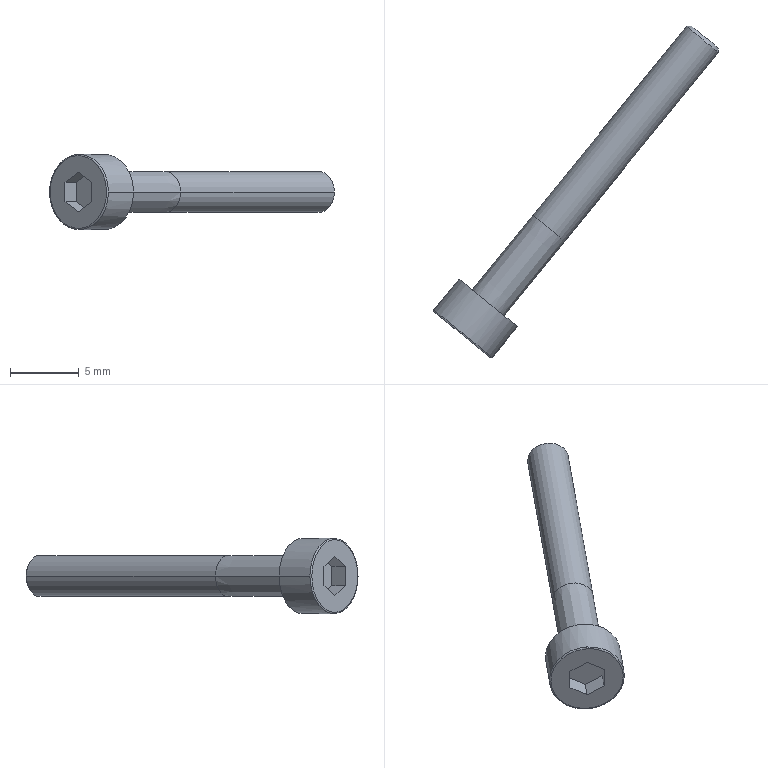Part | SolidWorks | features BaseBody 1 | 1 solid | 20 faces | box 20.765 x 24.207 x 5.5 mm | volume 240.606 mm3 | plane 10 | cylinder 4 | cone 4 | spline 2 | commonest cylinder face diameters 3 x2 5.5 x2
STEP:
#1=CARTESIAN_POINT('',(523.564,-199.626,281.731));
#2=VERTEX_POINT('',#1);
#3=CARTESIAN_POINT('',(525.697,-201.361,278.981));
#4=VERTEX_POINT('',#3);
#5=CARTESIAN_POINT('',(523.564,-199.626,278.981));
#6=DIRECTION('',(0.6309,0.7758,-0.000000012));
#7=DIRECTION('',(-0.7758,0.6309,0.));
#8=AXIS2_PLACEMENT_3D('',#5,#6,#7);
#9=CIRCLE('',#8,2.75);
#10=EDGE_CURVE('',#2,#4,#9,.T.);
#11=ORIENTED_EDGE('',*,*,#10,.F.);
#12=CARTESIAN_POINT('',(523.5,-199.704,281.631));
#13=VERTEX_POINT('',#12);
#14=CARTESIAN_POINT('',(523.564,-199.626,281.631));
#15=DIRECTION('',(0.7758,-0.6309,-0.000000021));
#16=DIRECTION('',(0.000000024,-0.000000004,1.));
#17=AXIS2_PLACEMENT_3D('',#14,#15,#16);
#18=CIRCLE('',#17,0.1);
#19=EDGE_CURVE('',#2,#13,#18,.T.);
#20=ORIENTED_EDGE('',*,*,#19,.T.);
#21=CARTESIAN_POINT('',(523.5,-199.704,276.331));
#22=VERTEX_POINT('',#21);
#23=CARTESIAN_POINT('',(523.5,-199.704,281.631));
#24=CARTESIAN_POINT('',(527.612,-203.048,281.631));
#25=CARTESIAN_POINT('',(527.612,-203.048,276.331));
#26=CARTESIAN_POINT('',(523.5,-199.704,276.331));
#27=(BOUNDED_CURVE()B_SPLINE_CURVE(3,(#23,#24,#25,#26),.UNSPECIFIED.,.F.,.F.)B_SPLINE_CURVE_WITH_KNOTS((4,4),(0.,1.),.UNSPECIFIED.)CURVE()GEOMETRIC_REPRESENTATION_ITEM()RATIONAL_B_SPLINE_CURVE((1.,0.3333,0.3333,1.))REPRESENTATION_ITEM(''));
#28=EDGE_CURVE('',#13,#22,#27,.T.);
#29=ORIENTED_EDGE('',*,*,#28,.T.);
#30=CARTESIAN_POINT('',(523.564,-199.626,276.231));
#31=VERTEX_POINT('',#30);
#32=CARTESIAN_POINT('',(523.564,-199.626,276.331));
#33=DIRECTION('',(-0.7758,0.6309,0.000000021));
#34=DIRECTION('',(-0.000000024,0.000000004,-1.));
#35=AXIS2_PLACEMENT_3D('',#32,#33,#34);
#36=CIRCLE('',#35,0.1);
#37=EDGE_CURVE('',#31,#22,#36,.T.);
#38=ORIENTED_EDGE('',*,*,#37,.F.);
#39=CARTESIAN_POINT('',(523.564,-199.626,278.981));
#40=DIRECTION('',(0.6309,0.7758,-0.000000012));
#41=DIRECTION('',(-0.7758,0.6309,0.));
#42=AXIS2_PLACEMENT_3D('',#39,#40,#41);
#43=CIRCLE('',#42,2.75);
#44=EDGE_CURVE('',#4,#31,#43,.T.);
#45=ORIENTED_EDGE('',*,*,#44,.F.);
#46=EDGE_LOOP('',(#11,#20,#29,#38,#45));
#47=FACE_OUTER_BOUND('',#46,.T.);
#48=CARTESIAN_POINT('',(523.564,-199.626,281.731));
#49=CARTESIAN_POINT('',(527.831,-203.097,281.731));
#50=CARTESIAN_POINT('',(527.831,-203.097,276.231));
#51=CARTESIAN_POINT('',(523.564,-199.626,276.231));
#52=CARTESIAN_POINT('',(523.527,-199.672,281.731));
#53=CARTESIAN_POINT('',(527.794,-203.142,281.731));
#54=CARTESIAN_POINT('',(527.794,-203.142,276.231));
#55=CARTESIAN_POINT('',(523.527,-199.672,276.231));
#56=CARTESIAN_POINT('',(523.5,-199.704,281.689));
#57=CARTESIAN_POINT('',(527.703,-203.122,281.689));
#58=CARTESIAN_POINT('',(527.703,-203.122,276.272));
#59=CARTESIAN_POINT('',(523.5,-199.704,276.272));
#60=CARTESIAN_POINT('',(523.5,-199.704,281.631));
#61=CARTESIAN_POINT('',(527.612,-203.048,281.631));
#62=CARTESIAN_POINT('',(527.612,-203.048,276.331));
#63=CARTESIAN_POINT('',(523.5,-199.704,276.331));
#64=(BOUNDED_SURFACE()B_SPLINE_SURFACE(3,3,((#48,#49,#50,#51),(#52,#53,#54,#55),(#56,#57,#58,#59),(#60,#61,#62,#63)),.UNSPECIFIED.,.F.,.F.,.T.)B_SPLINE_SURFACE_WITH_KNOTS((4,4),(4,4),(0.,1.),(0.,1.),.UNSPECIFIED.)GEOMETRIC_REPRESENTATION_ITEM()RATIONAL_B_SPLINE_SURFACE(((1.,0.3333,0.3333,1.),(0.8047,0.2682,0.2682,0.8047),(0.8047,0.2682,0.2682,0.8047),(1.,0.3333,0.3333,1.)))REPRESENTATION_ITEM('')SURFACE());
#65=ADVANCED_FACE('',(#47),#64,.T.);
#66=CARTESIAN_POINT('',(528.646,-190.999,278.981));
#67=VERTEX_POINT('',#66);
#68=CARTESIAN_POINT('',(530.974,-192.892,278.981));
#69=VERTEX_POINT('',#68);
#70=CARTESIAN_POINT('',(529.81,-191.946,278.981));
#71=DIRECTION('',(0.6309,0.7758,-0.000000012));
#72=DIRECTION('',(-0.7758,0.6309,0.));
#73=AXIS2_PLACEMENT_3D('',#70,#71,#72);
#74=CIRCLE('',#73,1.5);
#75=EDGE_CURVE('',#67,#69,#74,.T.);
#76=ORIENTED_EDGE('',*,*,#75,.T.);
#77=CARTESIAN_POINT('',(542.173,-179.121,278.981));
#78=VERTEX_POINT('',#77);
#79=CARTESIAN_POINT('',(536.573,-186.006,278.981));
#80=DIRECTION('',(0.6309,0.7758,-0.000000012));
#81=VECTOR('',#80,1000.);
#82=LINE('',#79,#81);
#83=EDGE_CURVE('',#69,#78,#82,.T.);
#84=ORIENTED_EDGE('',*,*,#83,.T.);
#85=CARTESIAN_POINT('',(539.845,-177.228,278.981));
#86=VERTEX_POINT('',#85);
#87=CARTESIAN_POINT('',(541.009,-178.174,278.981));
#88=DIRECTION('',(-0.6309,-0.7758,0.000000012));
#89=DIRECTION('',(-0.7758,0.6309,0.));
#90=AXIS2_PLACEMENT_3D('',#87,#88,#89);
#91=CIRCLE('',#90,1.5);
#92=EDGE_CURVE('',#78,#86,#91,.T.);
#93=ORIENTED_EDGE('',*,*,#92,.T.);
#94=CARTESIAN_POINT('',(534.246,-184.114,278.981));
#95=DIRECTION('',(0.6309,0.7758,-0.000000012));
#96=VECTOR('',#95,1000.);
#97=LINE('',#94,#96);
#98=EDGE_CURVE('',#67,#86,#97,.T.);
#99=ORIENTED_EDGE('',*,*,#98,.F.);
#100=EDGE_LOOP('',(#76,#84,#93,#99));
#101=FACE_OUTER_BOUND('',#100,.T.);
#102=CARTESIAN_POINT('',(535.409,-185.06,278.981));
#103=DIRECTION('',(0.6309,0.7758,-0.000000012));
#104=DIRECTION('',(-0.7758,0.6309,0.));
#105=AXIS2_PLACEMENT_3D('',#102,#103,#104);
#106=CYLINDRICAL_SURFACE('',#105,1.5);
#107=ADVANCED_FACE('',(#101),#106,.T.);
#108=CARTESIAN_POINT('',(542.136,-178.769,278.981));
#109=VERTEX_POINT('',#108);
#110=CARTESIAN_POINT('',(540.197,-177.192,278.981));
#111=VERTEX_POINT('',#110);
#112=CARTESIAN_POINT('',(541.167,-177.98,278.981));
#113=DIRECTION('',(-0.6309,-0.7758,0.000000012));
#114=DIRECTION('',(0.7758,-0.6309,0.));
#115=AXIS2_PLACEMENT_3D('',#112,#113,#114);
#116=CIRCLE('',#115,1.25);
#117=EDGE_CURVE('',#109,#111,#116,.T.);
#118=ORIENTED_EDGE('',*,*,#117,.T.);
#119=CARTESIAN_POINT('',(539.845,-177.228,278.981));
#120=DIRECTION('',(-0.9947,-0.1025,0.000000009));
#121=VECTOR('',#120,1000.);
#122=LINE('',#119,#121);
#123=EDGE_CURVE('',#111,#86,#122,.T.);
#124=ORIENTED_EDGE('',*,*,#123,.T.);
#125=ORIENTED_EDGE('',*,*,#92,.F.);
#126=CARTESIAN_POINT('',(542.173,-179.121,278.981));
#127=DIRECTION('',(0.1025,-0.9947,0.000000009));
#128=VECTOR('',#127,1000.);
#129=LINE('',#126,#128);
#130=EDGE_CURVE('',#109,#78,#129,.T.);
#131=ORIENTED_EDGE('',*,*,#130,.F.);
#132=EDGE_LOOP('',(#118,#124,#125,#131));
#133=FACE_OUTER_BOUND('',#132,.T.);
#134=CARTESIAN_POINT('',(541.009,-178.174,278.981));
#135=DIRECTION('',(-0.6309,-0.7758,0.000000012));
#136=DIRECTION('',(0.7758,-0.6309,0.));
#137=AXIS2_PLACEMENT_3D('',#134,#135,#136);
#138=CONICAL_SURFACE('',#137,1.5,0.7854);
#139=ADVANCED_FACE('',(#133),#138,.T.);
#140=CARTESIAN_POINT('',(524.23,-196.431,278.981));
#141=VERTEX_POINT('',#140);
#142=CARTESIAN_POINT('',(526.556,-198.322,278.981));
#143=VERTEX_POINT('',#142);
#144=CARTESIAN_POINT('',(525.393,-197.376,278.981));
#145=DIRECTION('',(0.6309,0.7758,-0.000000012));
#146=DIRECTION('',(-0.7758,0.6309,0.));
#147=AXIS2_PLACEMENT_3D('',#144,#145,#146);
#148=CIRCLE('',#147,1.499);
#149=EDGE_CURVE('',#141,#143,#148,.T.);
#150=ORIENTED_EDGE('',*,*,#149,.T.);
#151=CARTESIAN_POINT('',(530.974,-192.892,278.981));
#152=DIRECTION('',(0.631,0.7758,-0.000000012));
#153=VECTOR('',#152,1000.);
#154=LINE('',#151,#153);
#155=EDGE_CURVE('',#143,#69,#154,.T.);
#156=ORIENTED_EDGE('',*,*,#155,.T.);
#157=ORIENTED_EDGE('',*,*,#75,.F.);
#158=CARTESIAN_POINT('',(528.646,-190.999,278.981));
#159=DIRECTION('',(0.6308,0.7759,-0.000000012));
#160=VECTOR('',#159,1000.);
#161=LINE('',#158,#160);
#162=EDGE_CURVE('',#141,#67,#161,.T.);
#163=ORIENTED_EDGE('',*,*,#162,.F.);
#164=EDGE_LOOP('',(#150,#156,#157,#163));
#165=FACE_OUTER_BOUND('',#164,.T.);
#166=CARTESIAN_POINT('',(529.81,-191.946,278.981));
#167=DIRECTION('',(0.6309,0.7758,-0.000000012));
#168=DIRECTION('',(-0.7758,0.6309,0.));
#169=AXIS2_PLACEMENT_3D('',#166,#167,#168);
#170=CONICAL_SURFACE('',#169,1.5,0.0001071);
#171=ADVANCED_FACE('',(#165),#170,.T.);
#172=CARTESIAN_POINT('',(521.43,-197.891,278.981));
#173=VERTEX_POINT('',#172);
#174=CARTESIAN_POINT('',(523.564,-199.626,278.981));
#175=DIRECTION('',(0.6309,0.7758,-0.000000012));
#176=DIRECTION('',(-0.7758,0.6309,0.));
#177=AXIS2_PLACEMENT_3D('',#174,#175,#176);
#178=CIRCLE('',#177,2.75);
#179=EDGE_CURVE('',#173,#2,#178,.T.);
#180=ORIENTED_EDGE('',*,*,#179,.T.);
#181=ORIENTED_EDGE('',*,*,#10,.T.);
#182=CARTESIAN_POINT('',(527.527,-199.112,278.981));
#183=VERTEX_POINT('',#182);
#184=CARTESIAN_POINT('',(526.612,-200.236,278.981));
#185=DIRECTION('',(0.6309,0.7758,-0.000000012));
#186=VECTOR('',#185,1000.);
#187=LINE('',#184,#186);
#188=EDGE_CURVE('',#4,#183,#187,.T.);
#189=ORIENTED_EDGE('',*,*,#188,.T.);
#190=CARTESIAN_POINT('',(523.26,-195.641,278.981));
#191=VERTEX_POINT('',#190);
#192=CARTESIAN_POINT('',(525.393,-197.376,278.981));
#193=DIRECTION('',(0.6309,0.7758,-0.000000012));
#194=DIRECTION('',(-0.7758,0.6309,0.));
#195=AXIS2_PLACEMENT_3D('',#192,#193,#194);
#196=CIRCLE('',#195,2.75);
#197=EDGE_CURVE('',#191,#183,#196,.T.);
#198=ORIENTED_EDGE('',*,*,#197,.F.);
#199=CARTESIAN_POINT('',(522.345,-196.766,278.981));
#200=DIRECTION('',(0.6309,0.7758,-0.000000012));
#201=VECTOR('',#200,1000.);
#202=LINE('',#199,#201);
#203=EDGE_CURVE('',#173,#191,#202,.T.);
#204=ORIENTED_EDGE('',*,*,#203,.F.);
#205=EDGE_LOOP('',(#180,#181,#189,#198,#204));
#206=FACE_OUTER_BOUND('',#205,.T.);
#207=CARTESIAN_POINT('',(524.478,-198.501,278.981));
#208=DIRECTION('',(0.6309,0.7758,-0.000000012));
#209=DIRECTION('',(-0.7758,0.6309,0.));
#210=AXIS2_PLACEMENT_3D('',#207,#208,#209);
#211=CYLINDRICAL_SURFACE('',#210,2.75);
#212=ADVANCED_FACE('',(#206),#211,.T.);
#213=ORIENTED_EDGE('',*,*,#83,.F.);
#214=CARTESIAN_POINT('',(529.81,-191.946,278.981));
#215=DIRECTION('',(0.6309,0.7758,-0.000000012));
#216=DIRECTION('',(-0.7758,0.6309,0.));
#217=AXIS2_PLACEMENT_3D('',#214,#215,#216);
#218=CIRCLE('',#217,1.5);
#219=EDGE_CURVE('',#69,#67,#218,.T.);
#220=ORIENTED_EDGE('',*,*,#219,.T.);
#221=ORIENTED_EDGE('',*,*,#98,.T.);
#222=CARTESIAN_POINT('',(541.009,-178.174,278.981));
#223=DIRECTION('',(-0.6309,-0.7758,0.000000012));
#224=DIRECTION('',(-0.7758,0.6309,0.));
#225=AXIS2_PLACEMENT_3D('',#222,#223,#224);
#226=CIRCLE('',#225,1.5);
#227=EDGE_CURVE('',#86,#78,#226,.T.);
#228=ORIENTED_EDGE('',*,*,#227,.T.);
#229=EDGE_LOOP('',(#213,#220,#221,#228));
#230=FACE_OUTER_BOUND('',#229,.T.);
#231=CARTESIAN_POINT('',(535.409,-185.06,278.981));
#232=DIRECTION('',(0.6309,0.7758,-0.000000012));
#233=DIRECTION('',(-0.7758,0.6309,0.));
#234=AXIS2_PLACEMENT_3D('',#231,#232,#233);
#235=CYLINDRICAL_SURFACE('',#234,1.5);
#236=ADVANCED_FACE('',(#230),#235,.T.);
#237=ORIENTED_EDGE('',*,*,#123,.F.);
#238=CARTESIAN_POINT('',(541.167,-177.98,278.981));
#239=DIRECTION('',(-0.6309,-0.7758,0.000000012));
#240=DIRECTION('',(0.7758,-0.6309,0.));
#241=AXIS2_PLACEMENT_3D('',#238,#239,#240);
#242=CIRCLE('',#241,1.25);
#243=EDGE_CURVE('',#111,#109,#242,.T.);
#244=ORIENTED_EDGE('',*,*,#243,.T.);
#245=ORIENTED_EDGE('',*,*,#130,.T.);
#246=ORIENTED_EDGE('',*,*,#227,.F.);
#247=EDGE_LOOP('',(#237,#244,#245,#246));
#248=FACE_OUTER_BOUND('',#247,.T.);
#249=CARTESIAN_POINT('',(541.009,-178.174,278.981));
#250=DIRECTION('',(-0.6309,-0.7758,0.000000012));
#251=DIRECTION('',(0.7758,-0.6309,0.));
#252=AXIS2_PLACEMENT_3D('',#249,#250,#251);
#253=CONICAL_SURFACE('',#252,1.5,0.7854);
#254=ADVANCED_FACE('',(#248),#253,.T.);
#255=ORIENTED_EDGE('',*,*,#155,.F.);
#256=CARTESIAN_POINT('',(525.393,-197.376,278.981));
#257=DIRECTION('',(0.6309,0.7758,-0.000000012));
#258=DIRECTION('',(-0.7758,0.6309,0.));
#259=AXIS2_PLACEMENT_3D('',#256,#257,#258);
#260=CIRCLE('',#259,1.499);
#261=EDGE_CURVE('',#143,#141,#260,.T.);
#262=ORIENTED_EDGE('',*,*,#261,.T.);
#263=ORIENTED_EDGE('',*,*,#162,.T.);
#264=ORIENTED_EDGE('',*,*,#219,.F.);
#265=EDGE_LOOP('',(#255,#262,#263,#264));
#266=FACE_OUTER_BOUND('',#265,.T.);
#267=CARTESIAN_POINT('',(529.81,-191.946,278.981));
#268=DIRECTION('',(0.6309,0.7758,-0.000000012));
#269=DIRECTION('',(-0.7758,0.6309,0.));
#270=AXIS2_PLACEMENT_3D('',#267,#268,#269);
#271=CONICAL_SURFACE('',#270,1.5,0.0001071);
#272=ADVANCED_FACE('',(#266),#271,.T.);
#273=ORIENTED_EDGE('',*,*,#117,.F.);
#274=ORIENTED_EDGE('',*,*,#243,.F.);
#275=EDGE_LOOP('',(#273,#274));
#276=FACE_OUTER_BOUND('',#275,.T.);
#277=CARTESIAN_POINT('',(541.167,-177.98,278.356));
#278=DIRECTION('',(0.6309,0.7758,-0.000000012));
#279=DIRECTION('',(-0.7758,0.6309,0.));
#280=AXIS2_PLACEMENT_3D('',#277,#278,#279);
#281=PLANE('',#280);
#282=ADVANCED_FACE('',(#276),#281,.T.);
#283=ORIENTED_EDGE('',*,*,#149,.F.);
#284=ORIENTED_EDGE('',*,*,#261,.F.);
#285=EDGE_LOOP('',(#283,#284));
#286=FACE_BOUND('',#285,.T.);
#287=ORIENTED_EDGE('',*,*,#197,.T.);
#288=CARTESIAN_POINT('',(525.393,-197.376,278.981));
#289=DIRECTION('',(0.6309,0.7758,-0.000000012));
#290=DIRECTION('',(-0.7758,0.6309,0.));
#291=AXIS2_PLACEMENT_3D('',#288,#289,#290);
#292=CIRCLE('',#291,2.75);
#293=EDGE_CURVE('',#183,#191,#292,.T.);
#294=ORIENTED_EDGE('',*,*,#293,.T.);
#295=EDGE_LOOP('',(#287,#294));
#296=FACE_OUTER_BOUND('',#295,.T.);
#297=CARTESIAN_POINT('',(525.393,-197.376,277.606));
#298=DIRECTION('',(0.6309,0.7758,-0.000000012));
#299=DIRECTION('',(-0.7758,0.6309,0.));
#300=AXIS2_PLACEMENT_3D('',#297,#298,#299);
#301=PLANE('',#300);
#302=ADVANCED_FACE('',(#286,#296),#301,.T.);
#303=ORIENTED_EDGE('',*,*,#188,.F.);
#304=ORIENTED_EDGE('',*,*,#44,.T.);
#305=CARTESIAN_POINT('',(523.564,-199.626,278.981));
#306=DIRECTION('',(0.6309,0.7758,-0.000000012));
#307=DIRECTION('',(-0.7758,0.6309,0.));
#308=AXIS2_PLACEMENT_3D('',#305,#306,#307);
#309=CIRCLE('',#308,2.75);
#310=EDGE_CURVE('',#31,#173,#309,.T.);
#311=ORIENTED_EDGE('',*,*,#310,.T.);
#312=ORIENTED_EDGE('',*,*,#203,.T.);
#313=ORIENTED_EDGE('',*,*,#293,.F.);
#314=EDGE_LOOP('',(#303,#304,#311,#312,#313));
#315=FACE_OUTER_BOUND('',#314,.T.);
#316=CARTESIAN_POINT('',(524.478,-198.501,278.981));
#317=DIRECTION('',(0.6309,0.7758,-0.000000012));
#318=DIRECTION('',(-0.7758,0.6309,0.));
#319=AXIS2_PLACEMENT_3D('',#316,#317,#318);
#320=CYLINDRICAL_SURFACE('',#319,2.75);
#321=ADVANCED_FACE('',(#315),#320,.T.);
#322=ORIENTED_EDGE('',*,*,#19,.F.);
#323=ORIENTED_EDGE('',*,*,#179,.F.);
#324=ORIENTED_EDGE('',*,*,#310,.F.);
#325=ORIENTED_EDGE('',*,*,#37,.T.);
#326=CARTESIAN_POINT('',(523.5,-199.704,276.331));
#327=CARTESIAN_POINT('',(519.389,-196.36,276.331));
#328=CARTESIAN_POINT('',(519.389,-196.36,281.631));
#329=CARTESIAN_POINT('',(523.5,-199.704,281.631));
#330=(BOUNDED_CURVE()B_SPLINE_CURVE(3,(#326,#327,#328,#329),.UNSPECIFIED.,.F.,.F.)B_SPLINE_CURVE_WITH_KNOTS((4,4),(0.,1.),.UNSPECIFIED.)CURVE()GEOMETRIC_REPRESENTATION_ITEM()RATIONAL_B_SPLINE_CURVE((1.,0.3333,0.3333,1.))REPRESENTATION_ITEM(''));
#331=EDGE_CURVE('',#22,#13,#330,.T.);
#332=ORIENTED_EDGE('',*,*,#331,.T.);
#333=EDGE_LOOP('',(#322,#323,#324,#325,#332));
#334=FACE_OUTER_BOUND('',#333,.T.);
#335=CARTESIAN_POINT('',(523.564,-199.626,276.231));
#336=CARTESIAN_POINT('',(519.296,-196.156,276.231));
#337=CARTESIAN_POINT('',(519.296,-196.156,281.731));
#338=CARTESIAN_POINT('',(523.564,-199.626,281.731));
#339=CARTESIAN_POINT('',(523.527,-199.672,276.231));
#340=CARTESIAN_POINT('',(519.259,-196.202,276.231));
#341=CARTESIAN_POINT('',(519.259,-196.202,281.731));
#342=CARTESIAN_POINT('',(523.527,-199.672,281.731));
#343=CARTESIAN_POINT('',(523.5,-199.704,276.272));
#344=CARTESIAN_POINT('',(519.298,-196.286,276.272));
#345=CARTESIAN_POINT('',(519.298,-196.286,281.689));
#346=CARTESIAN_POINT('',(523.5,-199.704,281.689));
#347=CARTESIAN_POINT('',(523.5,-199.704,276.331));
#348=CARTESIAN_POINT('',(519.389,-196.36,276.331));
#349=CARTESIAN_POINT('',(519.389,-196.36,281.631));
#350=CARTESIAN_POINT('',(523.5,-199.704,281.631));
#351=(BOUNDED_SURFACE()B_SPLINE_SURFACE(3,3,((#335,#336,#337,#338),(#339,#340,#341,#342),(#343,#344,#345,#346),(#347,#348,#349,#350)),.UNSPECIFIED.,.F.,.F.,.F.)B_SPLINE_SURFACE_WITH_KNOTS((4,4),(4,4),(0.,1.),(0.,1.),.UNSPECIFIED.)GEOMETRIC_REPRESENTATION_ITEM()RATIONAL_B_SPLINE_SURFACE(((1.,0.3333,0.3333,1.),(0.8047,0.2682,0.2682,0.8047),(0.8047,0.2682,0.2682,0.8047),(1.,0.3333,0.3333,1.)))REPRESENTATION_ITEM('')SURFACE());
#352=ADVANCED_FACE('',(#334),#351,.T.);
#353=ORIENTED_EDGE('',*,*,#28,.F.);
#354=ORIENTED_EDGE('',*,*,#331,.F.);
#355=EDGE_LOOP('',(#353,#354));
#356=FACE_OUTER_BOUND('',#355,.T.);
#357=CARTESIAN_POINT('',(522.531,-198.915,279.702));
#358=VERTEX_POINT('',#357);
#359=CARTESIAN_POINT('',(523.5,-199.704,280.424));
#360=VERTEX_POINT('',#359);
#361=CARTESIAN_POINT('',(522.531,-198.915,279.702));
#362=DIRECTION('',(0.6719,-0.5464,0.5));
#363=VECTOR('',#362,1000.);
#364=LINE('',#361,#363);
#365=EDGE_CURVE('',#358,#360,#364,.T.);
#366=ORIENTED_EDGE('',*,*,#365,.T.);
#367=CARTESIAN_POINT('',(524.47,-200.493,279.702));
#368=VERTEX_POINT('',#367);
#369=CARTESIAN_POINT('',(523.5,-199.704,280.424));
#370=DIRECTION('',(0.6719,-0.5464,-0.5));
#371=VECTOR('',#370,1000.);
#372=LINE('',#369,#371);
#373=EDGE_CURVE('',#360,#368,#372,.T.);
#374=ORIENTED_EDGE('',*,*,#373,.T.);
#375=CARTESIAN_POINT('',(524.47,-200.493,278.259));
#376=VERTEX_POINT('',#375);
#377=CARTESIAN_POINT('',(524.47,-200.493,277.656));
#378=DIRECTION('',(-0.000000008,-0.000000009,-1.));
#379=VECTOR('',#378,1000.);
#380=LINE('',#377,#379);
#381=EDGE_CURVE('',#368,#376,#380,.T.);
#382=ORIENTED_EDGE('',*,*,#381,.T.);
#383=CARTESIAN_POINT('',(523.5,-199.704,277.537));
#384=VERTEX_POINT('',#383);
#385=CARTESIAN_POINT('',(524.47,-200.493,278.259));
#386=DIRECTION('',(-0.6719,0.5464,-0.5));
#387=VECTOR('',#386,1000.);
#388=LINE('',#385,#387);
#389=EDGE_CURVE('',#376,#384,#388,.T.);
#390=ORIENTED_EDGE('',*,*,#389,.T.);
#391=CARTESIAN_POINT('',(522.531,-198.915,278.259));
#392=VERTEX_POINT('',#391);
#393=CARTESIAN_POINT('',(523.5,-199.704,277.537));
#394=DIRECTION('',(-0.6719,0.5464,0.5));
#395=VECTOR('',#394,1000.);
#396=LINE('',#393,#395);
#397=EDGE_CURVE('',#384,#392,#396,.T.);
#398=ORIENTED_EDGE('',*,*,#397,.T.);
#399=CARTESIAN_POINT('',(522.531,-198.915,277.656));
#400=DIRECTION('',(0.000000008,0.000000009,1.));
#401=VECTOR('',#400,1000.);
#402=LINE('',#399,#401);
#403=EDGE_CURVE('',#392,#358,#402,.T.);
#404=ORIENTED_EDGE('',*,*,#403,.T.);
#405=EDGE_LOOP('',(#366,#374,#382,#390,#398,#404));
#406=FACE_BOUND('',#405,.T.);
#407=CARTESIAN_POINT('',(523.5,-199.704,277.656));
#408=DIRECTION('',(-0.6309,-0.7758,0.000000012));
#409=DIRECTION('',(0.7758,-0.6309,0.));
#410=AXIS2_PLACEMENT_3D('',#407,#408,#409);
#411=PLANE('',#410);
#412=ADVANCED_FACE('',(#356,#406),#411,.T.);
#413=CARTESIAN_POINT('',(525.29,-199.484,279.702));
#414=VERTEX_POINT('',#413);
#415=CARTESIAN_POINT('',(524.47,-200.493,279.702));
#416=DIRECTION('',(0.6309,0.7758,-0.000000012));
#417=VECTOR('',#416,1000.);
#418=LINE('',#415,#417);
#419=EDGE_CURVE('',#368,#414,#418,.T.);
#420=ORIENTED_EDGE('',*,*,#419,.F.);
#421=ORIENTED_EDGE('',*,*,#373,.F.);
#422=CARTESIAN_POINT('',(524.321,-198.695,280.424));
#423=VERTEX_POINT('',#422);
#424=CARTESIAN_POINT('',(524.321,-198.695,280.424));
#425=DIRECTION('',(-0.6309,-0.7758,0.000000012));
#426=VECTOR('',#425,1000.);
#427=LINE('',#424,#426);
#428=EDGE_CURVE('',#423,#360,#427,.T.);
#429=ORIENTED_EDGE('',*,*,#428,.F.);
#430=CARTESIAN_POINT('',(525.29,-199.484,279.702));
#431=DIRECTION('',(-0.6719,0.5464,0.5));
#432=VECTOR('',#431,1000.);
#433=LINE('',#430,#432);
#434=EDGE_CURVE('',#414,#423,#433,.T.);
#435=ORIENTED_EDGE('',*,*,#434,.F.);
#436=EDGE_LOOP('',(#420,#421,#429,#435));
#437=FACE_OUTER_BOUND('',#436,.T.);
#438=CARTESIAN_POINT('',(524.47,-200.493,279.702));
#439=DIRECTION('',(0.3879,-0.3155,0.866));
#440=DIRECTION('',(0.9126,0.,-0.4088));
#441=AXIS2_PLACEMENT_3D('',#438,#439,#440);
#442=PLANE('',#441);
#443=ADVANCED_FACE('',(#437),#442,.F.);
#444=ORIENTED_EDGE('',*,*,#428,.T.);
#445=ORIENTED_EDGE('',*,*,#365,.F.);
#446=CARTESIAN_POINT('',(523.351,-197.907,279.702));
#447=VERTEX_POINT('',#446);
#448=CARTESIAN_POINT('',(523.351,-197.907,279.702));
#449=DIRECTION('',(-0.6309,-0.7758,0.000000012));
#450=VECTOR('',#449,1000.);
#451=LINE('',#448,#450);
#452=EDGE_CURVE('',#447,#358,#451,.T.);
#453=ORIENTED_EDGE('',*,*,#452,.F.);
#454=CARTESIAN_POINT('',(524.321,-198.695,280.424));
#455=DIRECTION('',(-0.6719,0.5464,-0.5));
#456=VECTOR('',#455,1000.);
#457=LINE('',#454,#456);
#458=EDGE_CURVE('',#423,#447,#457,.T.);
#459=ORIENTED_EDGE('',*,*,#458,.F.);
#460=EDGE_LOOP('',(#444,#445,#453,#459));
#461=FACE_OUTER_BOUND('',#460,.T.);
#462=CARTESIAN_POINT('',(523.5,-199.704,280.424));
#463=DIRECTION('',(-0.3879,0.3155,0.866));
#464=DIRECTION('',(0.9126,0.,0.4088));
#465=AXIS2_PLACEMENT_3D('',#462,#463,#464);
#466=PLANE('',#465);
#467=ADVANCED_FACE('',(#461),#466,.F.);
#468=ORIENTED_EDGE('',*,*,#452,.T.);
#469=ORIENTED_EDGE('',*,*,#403,.F.);
#470=CARTESIAN_POINT('',(523.351,-197.907,278.259));
#471=VERTEX_POINT('',#470);
#472=CARTESIAN_POINT('',(522.531,-198.915,278.259));
#473=DIRECTION('',(-0.6309,-0.7758,0.));
#474=VECTOR('',#473,1000.);
#475=LINE('',#472,#474);
#476=EDGE_CURVE('',#471,#392,#475,.T.);
#477=ORIENTED_EDGE('',*,*,#476,.F.);
#478=CARTESIAN_POINT('',(523.351,-197.907,279.702));
#479=DIRECTION('',(-0.000000016,0.000000013,-1.));
#480=VECTOR('',#479,1000.);
#481=LINE('',#478,#480);
#482=EDGE_CURVE('',#447,#471,#481,.T.);
#483=ORIENTED_EDGE('',*,*,#482,.F.);
#484=EDGE_LOOP('',(#468,#469,#477,#483));
#485=FACE_OUTER_BOUND('',#484,.T.);
#486=CARTESIAN_POINT('',(522.531,-198.915,279.702));
#487=DIRECTION('',(-0.7758,0.6309,0.000000021));
#488=DIRECTION('',(-0.6309,-0.7758,0.));
#489=AXIS2_PLACEMENT_3D('',#486,#487,#488);
#490=PLANE('',#489);
#491=ADVANCED_FACE('',(#485),#490,.F.);
#492=ORIENTED_EDGE('',*,*,#476,.T.);
#493=ORIENTED_EDGE('',*,*,#397,.F.);
#494=CARTESIAN_POINT('',(524.321,-198.695,277.537));
#495=VERTEX_POINT('',#494);
#496=CARTESIAN_POINT('',(524.321,-198.695,277.537));
#497=DIRECTION('',(-0.6309,-0.7758,0.000000012));
#498=VECTOR('',#497,1000.);
#499=LINE('',#496,#498);
#500=EDGE_CURVE('',#495,#384,#499,.T.);
#501=ORIENTED_EDGE('',*,*,#500,.F.);
#502=CARTESIAN_POINT('',(523.351,-197.907,278.259));
#503=DIRECTION('',(0.6719,-0.5464,-0.5));
#504=VECTOR('',#503,1000.);
#505=LINE('',#502,#504);
#506=EDGE_CURVE('',#471,#495,#505,.T.);
#507=ORIENTED_EDGE('',*,*,#506,.F.);
#508=EDGE_LOOP('',(#492,#493,#501,#507));
#509=FACE_OUTER_BOUND('',#508,.T.);
#510=CARTESIAN_POINT('',(522.531,-198.915,278.259));
#511=DIRECTION('',(-0.3879,0.3155,-0.866));
#512=DIRECTION('',(-0.9126,0.,0.4088));
#513=AXIS2_PLACEMENT_3D('',#510,#511,#512);
#514=PLANE('',#513);
#515=ADVANCED_FACE('',(#509),#514,.F.);
#516=ORIENTED_EDGE('',*,*,#500,.T.);
#517=ORIENTED_EDGE('',*,*,#389,.F.);
#518=CARTESIAN_POINT('',(525.29,-199.484,278.259));
#519=VERTEX_POINT('',#518);
#520=CARTESIAN_POINT('',(525.29,-199.484,278.259));
#521=DIRECTION('',(-0.6309,-0.7758,0.000000012));
#522=VECTOR('',#521,1000.);
#523=LINE('',#520,#522);
#524=EDGE_CURVE('',#519,#376,#523,.T.);
#525=ORIENTED_EDGE('',*,*,#524,.F.);
#526=CARTESIAN_POINT('',(524.321,-198.695,277.537));
#527=DIRECTION('',(0.6719,-0.5464,0.5));
#528=VECTOR('',#527,1000.);
#529=LINE('',#526,#528);
#530=EDGE_CURVE('',#495,#519,#529,.T.);
#531=ORIENTED_EDGE('',*,*,#530,.F.);
#532=EDGE_LOOP('',(#516,#517,#525,#531));
#533=FACE_OUTER_BOUND('',#532,.T.);
#534=CARTESIAN_POINT('',(523.5,-199.704,277.537));
#535=DIRECTION('',(0.3879,-0.3155,-0.866));
#536=DIRECTION('',(-0.9126,0.,-0.4088));
#537=AXIS2_PLACEMENT_3D('',#534,#535,#536);
#538=PLANE('',#537);
#539=ADVANCED_FACE('',(#533),#538,.F.);
#540=ORIENTED_EDGE('',*,*,#524,.T.);
#541=ORIENTED_EDGE('',*,*,#381,.F.);
#542=ORIENTED_EDGE('',*,*,#419,.T.);
#543=CARTESIAN_POINT('',(525.29,-199.484,278.259));
#544=DIRECTION('',(0.000000016,-0.000000013,1.));
#545=VECTOR('',#544,1000.);
#546=LINE('',#543,#545);
#547=EDGE_CURVE('',#519,#414,#546,.T.);
#548=ORIENTED_EDGE('',*,*,#547,.F.);
#549=EDGE_LOOP('',(#540,#541,#542,#548));
#550=FACE_OUTER_BOUND('',#549,.T.);
#551=CARTESIAN_POINT('',(524.47,-200.493,278.259));
#552=DIRECTION('',(0.7758,-0.6309,-0.000000021));
#553=DIRECTION('',(0.6309,0.7758,0.));
#554=AXIS2_PLACEMENT_3D('',#551,#552,#553);
#555=PLANE('',#554);
#556=ADVANCED_FACE('',(#550),#555,.F.);
#557=ORIENTED_EDGE('',*,*,#506,.T.);
#558=ORIENTED_EDGE('',*,*,#530,.T.);
#559=ORIENTED_EDGE('',*,*,#547,.T.);
#560=ORIENTED_EDGE('',*,*,#434,.T.);
#561=ORIENTED_EDGE('',*,*,#458,.T.);
#562=ORIENTED_EDGE('',*,*,#482,.T.);
#563=EDGE_LOOP('',(#557,#558,#559,#560,#561,#562));
#564=FACE_OUTER_BOUND('',#563,.T.);
#565=CARTESIAN_POINT('',(524.321,-198.695,278.981));
#566=DIRECTION('',(-0.6309,-0.7758,0.000000012));
#567=DIRECTION('',(0.7758,-0.6309,0.));
#568=AXIS2_PLACEMENT_3D('',#565,#566,#567);
#569=PLANE('',#568);
#570=ADVANCED_FACE('',(#564),#569,.T.);
#571=CLOSED_SHELL('',(#65,#107,#139,#171,#212,#236,#254,#272,#282,#302,#321,#352,#412,#443,#467,#491,#515,#539,#556,#570));
#572=MANIFOLD_SOLID_BREP('',#571);
#573=CARTESIAN_POINT('',(0.,0.,0.));
#574=DIRECTION('',(0.,0.,1.));
#575=DIRECTION('',(1.,0.,0.));
#576=AXIS2_PLACEMENT_3D('',#573,#574,#575);
#577=(LENGTH_UNIT()NAMED_UNIT(*)SI_UNIT(.MILLI.,.METRE.));
#578=UNCERTAINTY_MEASURE_WITH_UNIT(LENGTH_MEASURE(0.00001),#577,'','');
#579=(NAMED_UNIT(*)PLANE_ANGLE_UNIT()SI_UNIT($,.RADIAN.));
#580=(NAMED_UNIT(*)SI_UNIT($,.STERADIAN.)SOLID_ANGLE_UNIT());
#581=(GEOMETRIC_REPRESENTATION_CONTEXT(3)GLOBAL_UNCERTAINTY_ASSIGNED_CONTEXT((#578))GLOBAL_UNIT_ASSIGNED_CONTEXT((#577,#579,#580))REPRESENTATION_CONTEXT('',''));
#582=ADVANCED_BREP_SHAPE_REPRESENTATION('',(#572,#576),#581);